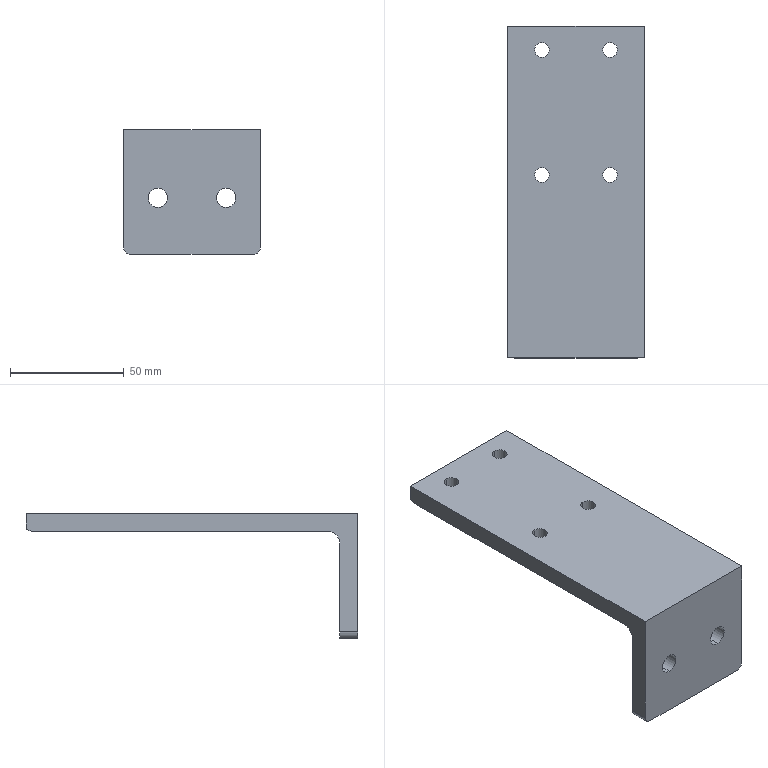Part | SolidWorks | features HoleWzd 2, ICE 2, 3DProfileFeature 1, Fillet 1, WeldMemberFeat 1, WeldmentFeature 1 | 1 solid | 24 faces | box 60 x 146 x 55 mm | volume 90878 mm3 | cylinder 16 | plane 8 | commonest cylinder face diameters 6.5 x8 8.5 x4 6 x2 10 x1 16 x1
STEP:
#1=CARTESIAN_POINT('',(15.,0.,-34.25));
#2=VERTEX_POINT('',#1);
#3=CARTESIAN_POINT('',(15.,0.,-25.75));
#4=VERTEX_POINT('',#3);
#5=CARTESIAN_POINT('',(15.,0.,-30.));
#6=DIRECTION('',(0.,1.,0.));
#7=DIRECTION('',(0.,0.,1.));
#8=AXIS2_PLACEMENT_3D('',#5,#6,#7);
#9=CIRCLE('',#8,4.25);
#10=EDGE_CURVE('',#2,#4,#9,.T.);
#11=ORIENTED_EDGE('',*,*,#10,.F.);
#12=CARTESIAN_POINT('',(15.,8.,-34.25));
#13=VERTEX_POINT('',#12);
#14=CARTESIAN_POINT('',(15.,8.,-34.25));
#15=DIRECTION('',(0.,1.,0.));
#16=VECTOR('',#15,1000.);
#17=LINE('',#14,#16);
#18=EDGE_CURVE('',#2,#13,#17,.T.);
#19=ORIENTED_EDGE('',*,*,#18,.T.);
#20=CARTESIAN_POINT('',(15.,8.,-25.75));
#21=VERTEX_POINT('',#20);
#22=CARTESIAN_POINT('',(15.,8.,-30.));
#23=DIRECTION('',(0.,1.,0.));
#24=DIRECTION('',(0.,0.,1.));
#25=AXIS2_PLACEMENT_3D('',#22,#23,#24);
#26=CIRCLE('',#25,4.25);
#27=EDGE_CURVE('',#13,#21,#26,.T.);
#28=ORIENTED_EDGE('',*,*,#27,.T.);
#29=CARTESIAN_POINT('',(15.,8.,-25.75));
#30=DIRECTION('',(0.,1.,0.));
#31=VECTOR('',#30,1000.);
#32=LINE('',#29,#31);
#33=EDGE_CURVE('',#4,#21,#32,.T.);
#34=ORIENTED_EDGE('',*,*,#33,.F.);
#35=EDGE_LOOP('',(#11,#19,#28,#34));
#36=FACE_OUTER_BOUND('',#35,.T.);
#37=CARTESIAN_POINT('',(15.,8.,-30.));
#38=DIRECTION('',(0.,1.,0.));
#39=DIRECTION('',(0.,0.,1.));
#40=AXIS2_PLACEMENT_3D('',#37,#38,#39);
#41=CYLINDRICAL_SURFACE('',#40,4.25);
#42=ADVANCED_FACE('',(#36),#41,.F.);
#43=CARTESIAN_POINT('',(45.,0.,-34.25));
#44=VERTEX_POINT('',#43);
#45=CARTESIAN_POINT('',(45.,0.,-25.75));
#46=VERTEX_POINT('',#45);
#47=CARTESIAN_POINT('',(45.,0.,-30.));
#48=DIRECTION('',(0.,1.,0.));
#49=DIRECTION('',(0.,0.,1.));
#50=AXIS2_PLACEMENT_3D('',#47,#48,#49);
#51=CIRCLE('',#50,4.25);
#52=EDGE_CURVE('',#44,#46,#51,.T.);
#53=ORIENTED_EDGE('',*,*,#52,.F.);
#54=CARTESIAN_POINT('',(45.,8.,-34.25));
#55=VERTEX_POINT('',#54);
#56=CARTESIAN_POINT('',(45.,8.,-34.25));
#57=DIRECTION('',(0.,1.,0.));
#58=VECTOR('',#57,1000.);
#59=LINE('',#56,#58);
#60=EDGE_CURVE('',#44,#55,#59,.T.);
#61=ORIENTED_EDGE('',*,*,#60,.T.);
#62=CARTESIAN_POINT('',(45.,8.,-25.75));
#63=VERTEX_POINT('',#62);
#64=CARTESIAN_POINT('',(45.,8.,-30.));
#65=DIRECTION('',(0.,1.,0.));
#66=DIRECTION('',(0.,0.,1.));
#67=AXIS2_PLACEMENT_3D('',#64,#65,#66);
#68=CIRCLE('',#67,4.25);
#69=EDGE_CURVE('',#55,#63,#68,.T.);
#70=ORIENTED_EDGE('',*,*,#69,.T.);
#71=CARTESIAN_POINT('',(45.,8.,-25.75));
#72=DIRECTION('',(0.,1.,0.));
#73=VECTOR('',#72,1000.);
#74=LINE('',#71,#73);
#75=EDGE_CURVE('',#46,#63,#74,.T.);
#76=ORIENTED_EDGE('',*,*,#75,.F.);
#77=EDGE_LOOP('',(#53,#61,#70,#76));
#78=FACE_OUTER_BOUND('',#77,.T.);
#79=CARTESIAN_POINT('',(45.,8.,-30.));
#80=DIRECTION('',(0.,1.,0.));
#81=DIRECTION('',(0.,0.,1.));
#82=AXIS2_PLACEMENT_3D('',#79,#80,#81);
#83=CYLINDRICAL_SURFACE('',#82,4.25);
#84=ADVANCED_FACE('',(#78),#83,.F.);
#85=CARTESIAN_POINT('',(45.,132.25,0.));
#86=VERTEX_POINT('',#85);
#87=CARTESIAN_POINT('',(45.,138.75,0.));
#88=VERTEX_POINT('',#87);
#89=CARTESIAN_POINT('',(45.,135.5,0.));
#90=DIRECTION('',(0.,0.,-1.));
#91=DIRECTION('',(0.,1.,0.));
#92=AXIS2_PLACEMENT_3D('',#89,#90,#91);
#93=CIRCLE('',#92,3.25);
#94=EDGE_CURVE('',#86,#88,#93,.T.);
#95=ORIENTED_EDGE('',*,*,#94,.F.);
#96=CARTESIAN_POINT('',(45.,132.25,-8.));
#97=VERTEX_POINT('',#96);
#98=CARTESIAN_POINT('',(45.,132.25,-8.));
#99=DIRECTION('',(0.,0.,-1.));
#100=VECTOR('',#99,1000.);
#101=LINE('',#98,#100);
#102=EDGE_CURVE('',#86,#97,#101,.T.);
#103=ORIENTED_EDGE('',*,*,#102,.T.);
#104=CARTESIAN_POINT('',(45.,138.75,-8.));
#105=VERTEX_POINT('',#104);
#106=CARTESIAN_POINT('',(45.,135.5,-8.));
#107=DIRECTION('',(0.,0.,-1.));
#108=DIRECTION('',(0.,1.,0.));
#109=AXIS2_PLACEMENT_3D('',#106,#107,#108);
#110=CIRCLE('',#109,3.25);
#111=EDGE_CURVE('',#97,#105,#110,.T.);
#112=ORIENTED_EDGE('',*,*,#111,.T.);
#113=CARTESIAN_POINT('',(45.,138.75,-8.));
#114=DIRECTION('',(0.,0.,-1.));
#115=VECTOR('',#114,1000.);
#116=LINE('',#113,#115);
#117=EDGE_CURVE('',#88,#105,#116,.T.);
#118=ORIENTED_EDGE('',*,*,#117,.F.);
#119=EDGE_LOOP('',(#95,#103,#112,#118));
#120=FACE_OUTER_BOUND('',#119,.T.);
#121=CARTESIAN_POINT('',(45.,135.5,-8.));
#122=DIRECTION('',(0.,0.,-1.));
#123=DIRECTION('',(0.,1.,0.));
#124=AXIS2_PLACEMENT_3D('',#121,#122,#123);
#125=CYLINDRICAL_SURFACE('',#124,3.25);
#126=ADVANCED_FACE('',(#120),#125,.F.);
#127=CARTESIAN_POINT('',(15.,132.25,0.));
#128=VERTEX_POINT('',#127);
#129=CARTESIAN_POINT('',(15.,138.75,0.));
#130=VERTEX_POINT('',#129);
#131=CARTESIAN_POINT('',(15.,135.5,0.));
#132=DIRECTION('',(0.,0.,-1.));
#133=DIRECTION('',(0.,1.,0.));
#134=AXIS2_PLACEMENT_3D('',#131,#132,#133);
#135=CIRCLE('',#134,3.25);
#136=EDGE_CURVE('',#128,#130,#135,.T.);
#137=ORIENTED_EDGE('',*,*,#136,.F.);
#138=CARTESIAN_POINT('',(15.,132.25,-8.));
#139=VERTEX_POINT('',#138);
#140=CARTESIAN_POINT('',(15.,132.25,-8.));
#141=DIRECTION('',(0.,0.,-1.));
#142=VECTOR('',#141,1000.);
#143=LINE('',#140,#142);
#144=EDGE_CURVE('',#128,#139,#143,.T.);
#145=ORIENTED_EDGE('',*,*,#144,.T.);
#146=CARTESIAN_POINT('',(15.,138.75,-8.));
#147=VERTEX_POINT('',#146);
#148=CARTESIAN_POINT('',(15.,135.5,-8.));
#149=DIRECTION('',(0.,0.,-1.));
#150=DIRECTION('',(0.,1.,0.));
#151=AXIS2_PLACEMENT_3D('',#148,#149,#150);
#152=CIRCLE('',#151,3.25);
#153=EDGE_CURVE('',#139,#147,#152,.T.);
#154=ORIENTED_EDGE('',*,*,#153,.T.);
#155=CARTESIAN_POINT('',(15.,138.75,-8.));
#156=DIRECTION('',(0.,0.,-1.));
#157=VECTOR('',#156,1000.);
#158=LINE('',#155,#157);
#159=EDGE_CURVE('',#130,#147,#158,.T.);
#160=ORIENTED_EDGE('',*,*,#159,.F.);
#161=EDGE_LOOP('',(#137,#145,#154,#160));
#162=FACE_OUTER_BOUND('',#161,.T.);
#163=CARTESIAN_POINT('',(15.,135.5,-8.));
#164=DIRECTION('',(0.,0.,-1.));
#165=DIRECTION('',(0.,1.,0.));
#166=AXIS2_PLACEMENT_3D('',#163,#164,#165);
#167=CYLINDRICAL_SURFACE('',#166,3.25);
#168=ADVANCED_FACE('',(#162),#167,.F.);
#169=CARTESIAN_POINT('',(45.,77.25,0.));
#170=VERTEX_POINT('',#169);
#171=CARTESIAN_POINT('',(45.,83.75,0.));
#172=VERTEX_POINT('',#171);
#173=CARTESIAN_POINT('',(45.,80.5,0.));
#174=DIRECTION('',(0.,0.,-1.));
#175=DIRECTION('',(0.,1.,0.));
#176=AXIS2_PLACEMENT_3D('',#173,#174,#175);
#177=CIRCLE('',#176,3.25);
#178=EDGE_CURVE('',#170,#172,#177,.T.);
#179=ORIENTED_EDGE('',*,*,#178,.F.);
#180=CARTESIAN_POINT('',(45.,77.25,-8.));
#181=VERTEX_POINT('',#180);
#182=CARTESIAN_POINT('',(45.,77.25,-8.));
#183=DIRECTION('',(0.,0.,-1.));
#184=VECTOR('',#183,1000.);
#185=LINE('',#182,#184);
#186=EDGE_CURVE('',#170,#181,#185,.T.);
#187=ORIENTED_EDGE('',*,*,#186,.T.);
#188=CARTESIAN_POINT('',(45.,83.75,-8.));
#189=VERTEX_POINT('',#188);
#190=CARTESIAN_POINT('',(45.,80.5,-8.));
#191=DIRECTION('',(0.,0.,-1.));
#192=DIRECTION('',(0.,1.,0.));
#193=AXIS2_PLACEMENT_3D('',#190,#191,#192);
#194=CIRCLE('',#193,3.25);
#195=EDGE_CURVE('',#181,#189,#194,.T.);
#196=ORIENTED_EDGE('',*,*,#195,.T.);
#197=CARTESIAN_POINT('',(45.,83.75,-8.));
#198=DIRECTION('',(0.,0.,-1.));
#199=VECTOR('',#198,1000.);
#200=LINE('',#197,#199);
#201=EDGE_CURVE('',#172,#189,#200,.T.);
#202=ORIENTED_EDGE('',*,*,#201,.F.);
#203=EDGE_LOOP('',(#179,#187,#196,#202));
#204=FACE_OUTER_BOUND('',#203,.T.);
#205=CARTESIAN_POINT('',(45.,80.5,-8.));
#206=DIRECTION('',(0.,0.,-1.));
#207=DIRECTION('',(0.,1.,0.));
#208=AXIS2_PLACEMENT_3D('',#205,#206,#207);
#209=CYLINDRICAL_SURFACE('',#208,3.25);
#210=ADVANCED_FACE('',(#204),#209,.F.);
#211=CARTESIAN_POINT('',(15.,77.25,0.));
#212=VERTEX_POINT('',#211);
#213=CARTESIAN_POINT('',(15.,83.75,0.));
#214=VERTEX_POINT('',#213);
#215=CARTESIAN_POINT('',(15.,80.5,0.));
#216=DIRECTION('',(0.,0.,-1.));
#217=DIRECTION('',(0.,1.,0.));
#218=AXIS2_PLACEMENT_3D('',#215,#216,#217);
#219=CIRCLE('',#218,3.25);
#220=EDGE_CURVE('',#212,#214,#219,.T.);
#221=ORIENTED_EDGE('',*,*,#220,.F.);
#222=CARTESIAN_POINT('',(15.,77.25,-8.));
#223=VERTEX_POINT('',#222);
#224=CARTESIAN_POINT('',(15.,77.25,-8.));
#225=DIRECTION('',(0.,0.,-1.));
#226=VECTOR('',#225,1000.);
#227=LINE('',#224,#226);
#228=EDGE_CURVE('',#212,#223,#227,.T.);
#229=ORIENTED_EDGE('',*,*,#228,.T.);
#230=CARTESIAN_POINT('',(15.,83.75,-8.));
#231=VERTEX_POINT('',#230);
#232=CARTESIAN_POINT('',(15.,80.5,-8.));
#233=DIRECTION('',(0.,0.,-1.));
#234=DIRECTION('',(0.,1.,0.));
#235=AXIS2_PLACEMENT_3D('',#232,#233,#234);
#236=CIRCLE('',#235,3.25);
#237=EDGE_CURVE('',#223,#231,#236,.T.);
#238=ORIENTED_EDGE('',*,*,#237,.T.);
#239=CARTESIAN_POINT('',(15.,83.75,-8.));
#240=DIRECTION('',(0.,0.,-1.));
#241=VECTOR('',#240,1000.);
#242=LINE('',#239,#241);
#243=EDGE_CURVE('',#214,#231,#242,.T.);
#244=ORIENTED_EDGE('',*,*,#243,.F.);
#245=EDGE_LOOP('',(#221,#229,#238,#244));
#246=FACE_OUTER_BOUND('',#245,.T.);
#247=CARTESIAN_POINT('',(15.,80.5,-8.));
#248=DIRECTION('',(0.,0.,-1.));
#249=DIRECTION('',(0.,1.,0.));
#250=AXIS2_PLACEMENT_3D('',#247,#248,#249);
#251=CYLINDRICAL_SURFACE('',#250,3.25);
#252=ADVANCED_FACE('',(#246),#251,.F.);
#253=CARTESIAN_POINT('',(45.,135.5,-8.));
#254=DIRECTION('',(0.,0.,-1.));
#255=DIRECTION('',(0.,1.,0.));
#256=AXIS2_PLACEMENT_3D('',#253,#254,#255);
#257=CIRCLE('',#256,3.25);
#258=EDGE_CURVE('',#105,#97,#257,.T.);
#259=ORIENTED_EDGE('',*,*,#258,.F.);
#260=ORIENTED_EDGE('',*,*,#111,.F.);
#261=EDGE_LOOP('',(#259,#260));
#262=FACE_BOUND('',#261,.T.);
#263=CARTESIAN_POINT('',(45.,80.5,-8.));
#264=DIRECTION('',(0.,0.,-1.));
#265=DIRECTION('',(0.,1.,0.));
#266=AXIS2_PLACEMENT_3D('',#263,#264,#265);
#267=CIRCLE('',#266,3.25);
#268=EDGE_CURVE('',#189,#181,#267,.T.);
#269=ORIENTED_EDGE('',*,*,#268,.F.);
#270=ORIENTED_EDGE('',*,*,#195,.F.);
#271=EDGE_LOOP('',(#269,#270));
#272=FACE_BOUND('',#271,.T.);
#273=CARTESIAN_POINT('',(15.,80.5,-8.));
#274=DIRECTION('',(0.,0.,-1.));
#275=DIRECTION('',(0.,1.,0.));
#276=AXIS2_PLACEMENT_3D('',#273,#274,#275);
#277=CIRCLE('',#276,3.25);
#278=EDGE_CURVE('',#231,#223,#277,.T.);
#279=ORIENTED_EDGE('',*,*,#278,.F.);
#280=ORIENTED_EDGE('',*,*,#237,.F.);
#281=EDGE_LOOP('',(#279,#280));
#282=FACE_BOUND('',#281,.T.);
#283=CARTESIAN_POINT('',(0.,13.,-8.));
#284=VERTEX_POINT('',#283);
#285=CARTESIAN_POINT('',(0.,142.,-8.));
#286=VERTEX_POINT('',#285);
#287=CARTESIAN_POINT('',(0.,142.,-8.));
#288=DIRECTION('',(0.,1.,0.));
#289=VECTOR('',#288,1000.);
#290=LINE('',#287,#289);
#291=EDGE_CURVE('',#284,#286,#290,.T.);
#292=ORIENTED_EDGE('',*,*,#291,.T.);
#293=CARTESIAN_POINT('',(60.,142.,-8.));
#294=VERTEX_POINT('',#293);
#295=CARTESIAN_POINT('',(60.,142.,-8.));
#296=DIRECTION('',(-1.,0.,0.));
#297=VECTOR('',#296,1000.);
#298=LINE('',#295,#297);
#299=EDGE_CURVE('',#294,#286,#298,.T.);
#300=ORIENTED_EDGE('',*,*,#299,.F.);
#301=CARTESIAN_POINT('',(60.,13.,-8.));
#302=VERTEX_POINT('',#301);
#303=CARTESIAN_POINT('',(60.,142.,-8.));
#304=DIRECTION('',(0.,1.,0.));
#305=VECTOR('',#304,1000.);
#306=LINE('',#303,#305);
#307=EDGE_CURVE('',#302,#294,#306,.T.);
#308=ORIENTED_EDGE('',*,*,#307,.F.);
#309=CARTESIAN_POINT('',(60.,13.,-8.));
#310=DIRECTION('',(-1.,0.,0.));
#311=VECTOR('',#310,1000.);
#312=LINE('',#309,#311);
#313=EDGE_CURVE('',#302,#284,#312,.T.);
#314=ORIENTED_EDGE('',*,*,#313,.T.);
#315=EDGE_LOOP('',(#292,#300,#308,#314));
#316=FACE_OUTER_BOUND('',#315,.T.);
#317=CARTESIAN_POINT('',(15.,135.5,-8.));
#318=DIRECTION('',(0.,0.,-1.));
#319=DIRECTION('',(0.,1.,0.));
#320=AXIS2_PLACEMENT_3D('',#317,#318,#319);
#321=CIRCLE('',#320,3.25);
#322=EDGE_CURVE('',#147,#139,#321,.T.);
#323=ORIENTED_EDGE('',*,*,#322,.F.);
#324=ORIENTED_EDGE('',*,*,#153,.F.);
#325=EDGE_LOOP('',(#323,#324));
#326=FACE_BOUND('',#325,.T.);
#327=CARTESIAN_POINT('',(60.,142.,-8.));
#328=DIRECTION('',(0.,0.,1.));
#329=DIRECTION('',(0.,-1.,0.));
#330=AXIS2_PLACEMENT_3D('',#327,#328,#329);
#331=PLANE('',#330);
#332=ADVANCED_FACE('',(#262,#272,#282,#316,#326),#331,.F.);
#333=CARTESIAN_POINT('',(15.,0.,-30.));
#334=DIRECTION('',(0.,1.,0.));
#335=DIRECTION('',(0.,0.,1.));
#336=AXIS2_PLACEMENT_3D('',#333,#334,#335);
#337=CIRCLE('',#336,4.25);
#338=EDGE_CURVE('',#4,#2,#337,.T.);
#339=ORIENTED_EDGE('',*,*,#338,.T.);
#340=ORIENTED_EDGE('',*,*,#10,.T.);
#341=EDGE_LOOP('',(#339,#340));
#342=FACE_BOUND('',#341,.T.);
#343=CARTESIAN_POINT('',(45.,0.,-30.));
#344=DIRECTION('',(0.,1.,0.));
#345=DIRECTION('',(0.,0.,1.));
#346=AXIS2_PLACEMENT_3D('',#343,#344,#345);
#347=CIRCLE('',#346,4.25);
#348=EDGE_CURVE('',#46,#44,#347,.T.);
#349=ORIENTED_EDGE('',*,*,#348,.T.);
#350=ORIENTED_EDGE('',*,*,#52,.T.);
#351=EDGE_LOOP('',(#349,#350));
#352=FACE_BOUND('',#351,.T.);
#353=CARTESIAN_POINT('',(0.,0.,0.));
#354=VERTEX_POINT('',#353);
#355=CARTESIAN_POINT('',(0.,0.,-52.));
#356=VERTEX_POINT('',#355);
#357=CARTESIAN_POINT('',(0.,0.,-70.));
#358=DIRECTION('',(0.,0.,-1.));
#359=VECTOR('',#358,1000.);
#360=LINE('',#357,#359);
#361=EDGE_CURVE('',#354,#356,#360,.T.);
#362=ORIENTED_EDGE('',*,*,#361,.T.);
#363=CARTESIAN_POINT('',(3.,0.,-55.));
#364=VERTEX_POINT('',#363);
#365=CARTESIAN_POINT('',(3.,0.,-52.));
#366=DIRECTION('',(0.,-1.,0.));
#367=DIRECTION('',(0.,0.,1.));
#368=AXIS2_PLACEMENT_3D('',#365,#366,#367);
#369=CIRCLE('',#368,3.);
#370=EDGE_CURVE('',#356,#364,#369,.T.);
#371=ORIENTED_EDGE('',*,*,#370,.T.);
#372=CARTESIAN_POINT('',(57.,0.,-55.));
#373=VERTEX_POINT('',#372);
#374=CARTESIAN_POINT('',(0.,0.,-55.));
#375=DIRECTION('',(-1.,0.,0.));
#376=VECTOR('',#375,1000.);
#377=LINE('',#374,#376);
#378=EDGE_CURVE('',#373,#364,#377,.T.);
#379=ORIENTED_EDGE('',*,*,#378,.F.);
#380=CARTESIAN_POINT('',(60.,0.,-52.));
#381=VERTEX_POINT('',#380);
#382=CARTESIAN_POINT('',(57.,0.,-52.));
#383=DIRECTION('',(0.,-1.,0.));
#384=DIRECTION('',(0.,0.,1.));
#385=AXIS2_PLACEMENT_3D('',#382,#383,#384);
#386=CIRCLE('',#385,3.);
#387=EDGE_CURVE('',#373,#381,#386,.T.);
#388=ORIENTED_EDGE('',*,*,#387,.T.);
#389=CARTESIAN_POINT('',(60.,0.,0.));
#390=VERTEX_POINT('',#389);
#391=CARTESIAN_POINT('',(60.,0.,-70.));
#392=DIRECTION('',(0.,0.,-1.));
#393=VECTOR('',#392,1000.);
#394=LINE('',#391,#393);
#395=EDGE_CURVE('',#390,#381,#394,.T.);
#396=ORIENTED_EDGE('',*,*,#395,.F.);
#397=CARTESIAN_POINT('',(60.,0.,0.));
#398=DIRECTION('',(-1.,0.,0.));
#399=VECTOR('',#398,1000.);
#400=LINE('',#397,#399);
#401=EDGE_CURVE('',#390,#354,#400,.T.);
#402=ORIENTED_EDGE('',*,*,#401,.T.);
#403=EDGE_LOOP('',(#362,#371,#379,#388,#396,#402));
#404=FACE_OUTER_BOUND('',#403,.T.);
#405=CARTESIAN_POINT('',(60.,0.,-70.));
#406=DIRECTION('',(0.,1.,0.));
#407=DIRECTION('',(0.,0.,1.));
#408=AXIS2_PLACEMENT_3D('',#405,#406,#407);
#409=PLANE('',#408);
#410=ADVANCED_FACE('',(#342,#352,#404),#409,.F.);
#411=CARTESIAN_POINT('',(15.,8.,-30.));
#412=DIRECTION('',(0.,1.,0.));
#413=DIRECTION('',(0.,0.,1.));
#414=AXIS2_PLACEMENT_3D('',#411,#412,#413);
#415=CIRCLE('',#414,4.25);
#416=EDGE_CURVE('',#21,#13,#415,.T.);
#417=ORIENTED_EDGE('',*,*,#416,.F.);
#418=ORIENTED_EDGE('',*,*,#27,.F.);
#419=EDGE_LOOP('',(#417,#418));
#420=FACE_BOUND('',#419,.T.);
#421=CARTESIAN_POINT('',(45.,8.,-30.));
#422=DIRECTION('',(0.,1.,0.));
#423=DIRECTION('',(0.,0.,1.));
#424=AXIS2_PLACEMENT_3D('',#421,#422,#423);
#425=CIRCLE('',#424,4.25);
#426=EDGE_CURVE('',#63,#55,#425,.T.);
#427=ORIENTED_EDGE('',*,*,#426,.F.);
#428=ORIENTED_EDGE('',*,*,#69,.F.);
#429=EDGE_LOOP('',(#427,#428));
#430=FACE_BOUND('',#429,.T.);
#431=CARTESIAN_POINT('',(57.,8.,-55.));
#432=VERTEX_POINT('',#431);
#433=CARTESIAN_POINT('',(3.,8.,-55.));
#434=VERTEX_POINT('',#433);
#435=CARTESIAN_POINT('',(60.,8.,-55.));
#436=DIRECTION('',(-1.,0.,0.));
#437=VECTOR('',#436,1000.);
#438=LINE('',#435,#437);
#439=EDGE_CURVE('',#432,#434,#438,.T.);
#440=ORIENTED_EDGE('',*,*,#439,.T.);
#441=CARTESIAN_POINT('',(0.,8.,-52.));
#442=VERTEX_POINT('',#441);
#443=CARTESIAN_POINT('',(3.,8.,-52.));
#444=DIRECTION('',(0.,1.,0.));
#445=DIRECTION('',(0.,0.,-1.));
#446=AXIS2_PLACEMENT_3D('',#443,#444,#445);
#447=CIRCLE('',#446,3.);
#448=EDGE_CURVE('',#434,#442,#447,.T.);
#449=ORIENTED_EDGE('',*,*,#448,.T.);
#450=CARTESIAN_POINT('',(0.,8.,-13.));
#451=VERTEX_POINT('',#450);
#452=CARTESIAN_POINT('',(0.,8.,-13.));
#453=DIRECTION('',(0.,0.,1.));
#454=VECTOR('',#453,1000.);
#455=LINE('',#452,#454);
#456=EDGE_CURVE('',#442,#451,#455,.T.);
#457=ORIENTED_EDGE('',*,*,#456,.T.);
#458=CARTESIAN_POINT('',(60.,8.,-13.));
#459=VERTEX_POINT('',#458);
#460=CARTESIAN_POINT('',(60.,8.,-13.));
#461=DIRECTION('',(-1.,0.,0.));
#462=VECTOR('',#461,1000.);
#463=LINE('',#460,#462);
#464=EDGE_CURVE('',#459,#451,#463,.T.);
#465=ORIENTED_EDGE('',*,*,#464,.F.);
#466=CARTESIAN_POINT('',(60.,8.,-52.));
#467=VERTEX_POINT('',#466);
#468=CARTESIAN_POINT('',(60.,8.,-13.));
#469=DIRECTION('',(0.,0.,1.));
#470=VECTOR('',#469,1000.);
#471=LINE('',#468,#470);
#472=EDGE_CURVE('',#467,#459,#471,.T.);
#473=ORIENTED_EDGE('',*,*,#472,.F.);
#474=CARTESIAN_POINT('',(57.,8.,-52.));
#475=DIRECTION('',(0.,1.,0.));
#476=DIRECTION('',(0.,0.,-1.));
#477=AXIS2_PLACEMENT_3D('',#474,#475,#476);
#478=CIRCLE('',#477,3.);
#479=EDGE_CURVE('',#467,#432,#478,.T.);
#480=ORIENTED_EDGE('',*,*,#479,.T.);
#481=EDGE_LOOP('',(#440,#449,#457,#465,#473,#480));
#482=FACE_OUTER_BOUND('',#481,.T.);
#483=CARTESIAN_POINT('',(60.,8.,-13.));
#484=DIRECTION('',(0.,-1.,0.));
#485=DIRECTION('',(0.,0.,-1.));
#486=AXIS2_PLACEMENT_3D('',#483,#484,#485);
#487=PLANE('',#486);
#488=ADVANCED_FACE('',(#420,#430,#482),#487,.F.);
#489=CARTESIAN_POINT('',(0.,13.,-13.));
#490=DIRECTION('',(-1.,0.,0.));
#491=DIRECTION('',(0.,0.,1.));
#492=AXIS2_PLACEMENT_3D('',#489,#490,#491);
#493=CIRCLE('',#492,5.);
#494=EDGE_CURVE('',#451,#284,#493,.T.);
#495=ORIENTED_EDGE('',*,*,#494,.T.);
#496=ORIENTED_EDGE('',*,*,#313,.F.);
#497=CARTESIAN_POINT('',(60.,13.,-13.));
#498=DIRECTION('',(-1.,0.,0.));
#499=DIRECTION('',(0.,0.,1.));
#500=AXIS2_PLACEMENT_3D('',#497,#498,#499);
#501=CIRCLE('',#500,5.);
#502=EDGE_CURVE('',#459,#302,#501,.T.);
#503=ORIENTED_EDGE('',*,*,#502,.F.);
#504=ORIENTED_EDGE('',*,*,#464,.T.);
#505=EDGE_LOOP('',(#495,#496,#503,#504));
#506=FACE_OUTER_BOUND('',#505,.T.);
#507=CARTESIAN_POINT('',(60.,13.,-13.));
#508=DIRECTION('',(-1.,0.,0.));
#509=DIRECTION('',(0.,0.,1.));
#510=AXIS2_PLACEMENT_3D('',#507,#508,#509);
#511=CYLINDRICAL_SURFACE('',#510,5.);
#512=ADVANCED_FACE('',(#506),#511,.F.);
#513=CARTESIAN_POINT('',(0.,146.,-6.928));
#514=VERTEX_POINT('',#513);
#515=CARTESIAN_POINT('',(0.,142.,0.));
#516=DIRECTION('',(1.,0.,0.));
#517=DIRECTION('',(0.,0.,1.));
#518=AXIS2_PLACEMENT_3D('',#515,#516,#517);
#519=CIRCLE('',#518,8.);
#520=EDGE_CURVE('',#286,#514,#519,.T.);
#521=ORIENTED_EDGE('',*,*,#520,.T.);
#522=CARTESIAN_POINT('',(60.,146.,-6.928));
#523=VERTEX_POINT('',#522);
#524=CARTESIAN_POINT('',(60.,146.,-6.928));
#525=DIRECTION('',(1.,0.,0.));
#526=VECTOR('',#525,1000.);
#527=LINE('',#524,#526);
#528=EDGE_CURVE('',#514,#523,#527,.T.);
#529=ORIENTED_EDGE('',*,*,#528,.T.);
#530=CARTESIAN_POINT('',(60.,142.,0.));
#531=DIRECTION('',(1.,0.,0.));
#532=DIRECTION('',(0.,0.,1.));
#533=AXIS2_PLACEMENT_3D('',#530,#531,#532);
#534=CIRCLE('',#533,8.);
#535=EDGE_CURVE('',#294,#523,#534,.T.);
#536=ORIENTED_EDGE('',*,*,#535,.F.);
#537=ORIENTED_EDGE('',*,*,#299,.T.);
#538=EDGE_LOOP('',(#521,#529,#536,#537));
#539=FACE_OUTER_BOUND('',#538,.T.);
#540=CARTESIAN_POINT('',(60.,142.,0.));
#541=DIRECTION('',(-1.,0.,0.));
#542=DIRECTION('',(0.,0.,1.));
#543=AXIS2_PLACEMENT_3D('',#540,#541,#542);
#544=CYLINDRICAL_SURFACE('',#543,8.);
#545=ADVANCED_FACE('',(#539),#544,.T.);
#546=CARTESIAN_POINT('',(45.,135.5,0.));
#547=DIRECTION('',(0.,0.,-1.));
#548=DIRECTION('',(0.,1.,0.));
#549=AXIS2_PLACEMENT_3D('',#546,#547,#548);
#550=CIRCLE('',#549,3.25);
#551=EDGE_CURVE('',#88,#86,#550,.T.);
#552=ORIENTED_EDGE('',*,*,#551,.T.);
#553=ORIENTED_EDGE('',*,*,#94,.T.);
#554=EDGE_LOOP('',(#552,#553));
#555=FACE_BOUND('',#554,.T.);
#556=CARTESIAN_POINT('',(15.,135.5,0.));
#557=DIRECTION('',(0.,0.,-1.));
#558=DIRECTION('',(0.,1.,0.));
#559=AXIS2_PLACEMENT_3D('',#556,#557,#558);
#560=CIRCLE('',#559,3.25);
#561=EDGE_CURVE('',#130,#128,#560,.T.);
#562=ORIENTED_EDGE('',*,*,#561,.T.);
#563=ORIENTED_EDGE('',*,*,#136,.T.);
#564=EDGE_LOOP('',(#562,#563));
#565=FACE_BOUND('',#564,.T.);
#566=CARTESIAN_POINT('',(45.,80.5,0.));
#567=DIRECTION('',(0.,0.,-1.));
#568=DIRECTION('',(0.,1.,0.));
#569=AXIS2_PLACEMENT_3D('',#566,#567,#568);
#570=CIRCLE('',#569,3.25);
#571=EDGE_CURVE('',#172,#170,#570,.T.);
#572=ORIENTED_EDGE('',*,*,#571,.T.);
#573=ORIENTED_EDGE('',*,*,#178,.T.);
#574=EDGE_LOOP('',(#572,#573));
#575=FACE_BOUND('',#574,.T.);
#576=CARTESIAN_POINT('',(15.,80.5,0.));
#577=DIRECTION('',(0.,0.,-1.));
#578=DIRECTION('',(0.,1.,0.));
#579=AXIS2_PLACEMENT_3D('',#576,#577,#578);
#580=CIRCLE('',#579,3.25);
#581=EDGE_CURVE('',#214,#212,#580,.T.);
#582=ORIENTED_EDGE('',*,*,#581,.T.);
#583=ORIENTED_EDGE('',*,*,#220,.T.);
#584=EDGE_LOOP('',(#582,#583));
#585=FACE_BOUND('',#584,.T.);
#586=CARTESIAN_POINT('',(60.,146.,0.));
#587=VERTEX_POINT('',#586);
#588=CARTESIAN_POINT('',(60.,0.,0.));
#589=DIRECTION('',(0.,-1.,0.));
#590=VECTOR('',#589,1000.);
#591=LINE('',#588,#590);
#592=EDGE_CURVE('',#587,#390,#591,.T.);
#593=ORIENTED_EDGE('',*,*,#592,.F.);
#594=CARTESIAN_POINT('',(0.,146.,0.));
#595=VERTEX_POINT('',#594);
#596=CARTESIAN_POINT('',(60.,146.,0.));
#597=DIRECTION('',(1.,0.,0.));
#598=VECTOR('',#597,1000.);
#599=LINE('',#596,#598);
#600=EDGE_CURVE('',#595,#587,#599,.T.);
#601=ORIENTED_EDGE('',*,*,#600,.F.);
#602=CARTESIAN_POINT('',(0.,0.,0.));
#603=DIRECTION('',(0.,-1.,0.));
#604=VECTOR('',#603,1000.);
#605=LINE('',#602,#604);
#606=EDGE_CURVE('',#595,#354,#605,.T.);
#607=ORIENTED_EDGE('',*,*,#606,.T.);
#608=ORIENTED_EDGE('',*,*,#401,.F.);
#609=EDGE_LOOP('',(#593,#601,#607,#608));
#610=FACE_OUTER_BOUND('',#609,.T.);
#611=CARTESIAN_POINT('',(60.,0.,0.));
#612=DIRECTION('',(0.,0.,-1.));
#613=DIRECTION('',(-1.,0.,0.));
#614=AXIS2_PLACEMENT_3D('',#611,#612,#613);
#615=PLANE('',#614);
#616=ADVANCED_FACE('',(#555,#565,#575,#585,#610),#615,.F.);
#617=ORIENTED_EDGE('',*,*,#395,.T.);
#618=CARTESIAN_POINT('',(60.,142.,-52.));
#619=DIRECTION('',(0.,1.,0.));
#620=VECTOR('',#619,1000.);
#621=LINE('',#618,#620);
#622=EDGE_CURVE('',#381,#467,#621,.T.);
#623=ORIENTED_EDGE('',*,*,#622,.T.);
#624=ORIENTED_EDGE('',*,*,#472,.T.);
#625=ORIENTED_EDGE('',*,*,#502,.T.);
#626=ORIENTED_EDGE('',*,*,#307,.T.);
#627=ORIENTED_EDGE('',*,*,#535,.T.);
#628=CARTESIAN_POINT('',(60.,146.,-55.));
#629=DIRECTION('',(0.,0.,1.));
#630=VECTOR('',#629,1000.);
#631=LINE('',#628,#630);
#632=EDGE_CURVE('',#523,#587,#631,.T.);
#633=ORIENTED_EDGE('',*,*,#632,.T.);
#634=ORIENTED_EDGE('',*,*,#592,.T.);
#635=EDGE_LOOP('',(#617,#623,#624,#625,#626,#627,#633,#634));
#636=FACE_OUTER_BOUND('',#635,.T.);
#637=CARTESIAN_POINT('',(60.,142.,0.));
#638=DIRECTION('',(-1.,0.,0.));
#639=DIRECTION('',(0.,0.,1.));
#640=AXIS2_PLACEMENT_3D('',#637,#638,#639);
#641=PLANE('',#640);
#642=ADVANCED_FACE('',(#636),#641,.F.);
#643=ORIENTED_EDGE('',*,*,#456,.F.);
#644=CARTESIAN_POINT('',(0.,0.,-52.));
#645=DIRECTION('',(0.,-1.,0.));
#646=VECTOR('',#645,1000.);
#647=LINE('',#644,#646);
#648=EDGE_CURVE('',#442,#356,#647,.T.);
#649=ORIENTED_EDGE('',*,*,#648,.T.);
#650=ORIENTED_EDGE('',*,*,#361,.F.);
#651=ORIENTED_EDGE('',*,*,#606,.F.);
#652=CARTESIAN_POINT('',(0.,146.,0.));
#653=DIRECTION('',(0.,0.,1.));
#654=VECTOR('',#653,1000.);
#655=LINE('',#652,#654);
#656=EDGE_CURVE('',#514,#595,#655,.T.);
#657=ORIENTED_EDGE('',*,*,#656,.F.);
#658=ORIENTED_EDGE('',*,*,#520,.F.);
#659=ORIENTED_EDGE('',*,*,#291,.F.);
#660=ORIENTED_EDGE('',*,*,#494,.F.);
#661=EDGE_LOOP('',(#643,#649,#650,#651,#657,#658,#659,#660));
#662=FACE_OUTER_BOUND('',#661,.T.);
#663=CARTESIAN_POINT('',(0.,142.,0.));
#664=DIRECTION('',(-1.,0.,0.));
#665=DIRECTION('',(0.,0.,1.));
#666=AXIS2_PLACEMENT_3D('',#663,#664,#665);
#667=PLANE('',#666);
#668=ADVANCED_FACE('',(#662),#667,.T.);
#669=ORIENTED_EDGE('',*,*,#378,.T.);
#670=CARTESIAN_POINT('',(3.,8.,-55.));
#671=DIRECTION('',(0.,1.,0.));
#672=VECTOR('',#671,1000.);
#673=LINE('',#670,#672);
#674=EDGE_CURVE('',#364,#434,#673,.T.);
#675=ORIENTED_EDGE('',*,*,#674,.T.);
#676=ORIENTED_EDGE('',*,*,#439,.F.);
#677=CARTESIAN_POINT('',(57.,150.,-55.));
#678=DIRECTION('',(0.,-1.,0.));
#679=VECTOR('',#678,1000.);
#680=LINE('',#677,#679);
#681=EDGE_CURVE('',#432,#373,#680,.T.);
#682=ORIENTED_EDGE('',*,*,#681,.T.);
#683=EDGE_LOOP('',(#669,#675,#676,#682));
#684=FACE_OUTER_BOUND('',#683,.T.);
#685=CARTESIAN_POINT('',(0.,150.,-55.));
#686=DIRECTION('',(0.,0.,1.));
#687=DIRECTION('',(1.,0.,0.));
#688=AXIS2_PLACEMENT_3D('',#685,#686,#687);
#689=PLANE('',#688);
#690=ADVANCED_FACE('',(#684),#689,.F.);
#691=ORIENTED_EDGE('',*,*,#656,.T.);
#692=ORIENTED_EDGE('',*,*,#600,.T.);
#693=ORIENTED_EDGE('',*,*,#632,.F.);
#694=ORIENTED_EDGE('',*,*,#528,.F.);
#695=EDGE_LOOP('',(#691,#692,#693,#694));
#696=FACE_OUTER_BOUND('',#695,.T.);
#697=CARTESIAN_POINT('',(60.,146.,-55.));
#698=DIRECTION('',(0.,-1.,0.));
#699=DIRECTION('',(0.,0.,-1.));
#700=AXIS2_PLACEMENT_3D('',#697,#698,#699);
#701=PLANE('',#700);
#702=ADVANCED_FACE('',(#696),#701,.F.);
#703=ORIENTED_EDGE('',*,*,#228,.F.);
#704=ORIENTED_EDGE('',*,*,#581,.F.);
#705=ORIENTED_EDGE('',*,*,#243,.T.);
#706=ORIENTED_EDGE('',*,*,#278,.T.);
#707=EDGE_LOOP('',(#703,#704,#705,#706));
#708=FACE_OUTER_BOUND('',#707,.T.);
#709=CARTESIAN_POINT('',(15.,80.5,-8.));
#710=DIRECTION('',(0.,0.,-1.));
#711=DIRECTION('',(0.,1.,0.));
#712=AXIS2_PLACEMENT_3D('',#709,#710,#711);
#713=CYLINDRICAL_SURFACE('',#712,3.25);
#714=ADVANCED_FACE('',(#708),#713,.F.);
#715=ORIENTED_EDGE('',*,*,#186,.F.);
#716=ORIENTED_EDGE('',*,*,#571,.F.);
#717=ORIENTED_EDGE('',*,*,#201,.T.);
#718=ORIENTED_EDGE('',*,*,#268,.T.);
#719=EDGE_LOOP('',(#715,#716,#717,#718));
#720=FACE_OUTER_BOUND('',#719,.T.);
#721=CARTESIAN_POINT('',(45.,80.5,-8.));
#722=DIRECTION('',(0.,0.,-1.));
#723=DIRECTION('',(0.,1.,0.));
#724=AXIS2_PLACEMENT_3D('',#721,#722,#723);
#725=CYLINDRICAL_SURFACE('',#724,3.25);
#726=ADVANCED_FACE('',(#720),#725,.F.);
#727=ORIENTED_EDGE('',*,*,#144,.F.);
#728=ORIENTED_EDGE('',*,*,#561,.F.);
#729=ORIENTED_EDGE('',*,*,#159,.T.);
#730=ORIENTED_EDGE('',*,*,#322,.T.);
#731=EDGE_LOOP('',(#727,#728,#729,#730));
#732=FACE_OUTER_BOUND('',#731,.T.);
#733=CARTESIAN_POINT('',(15.,135.5,-8.));
#734=DIRECTION('',(0.,0.,-1.));
#735=DIRECTION('',(0.,1.,0.));
#736=AXIS2_PLACEMENT_3D('',#733,#734,#735);
#737=CYLINDRICAL_SURFACE('',#736,3.25);
#738=ADVANCED_FACE('',(#732),#737,.F.);
#739=ORIENTED_EDGE('',*,*,#102,.F.);
#740=ORIENTED_EDGE('',*,*,#551,.F.);
#741=ORIENTED_EDGE('',*,*,#117,.T.);
#742=ORIENTED_EDGE('',*,*,#258,.T.);
#743=EDGE_LOOP('',(#739,#740,#741,#742));
#744=FACE_OUTER_BOUND('',#743,.T.);
#745=CARTESIAN_POINT('',(45.,135.5,-8.));
#746=DIRECTION('',(0.,0.,-1.));
#747=DIRECTION('',(0.,1.,0.));
#748=AXIS2_PLACEMENT_3D('',#745,#746,#747);
#749=CYLINDRICAL_SURFACE('',#748,3.25);
#750=ADVANCED_FACE('',(#744),#749,.F.);
#751=ORIENTED_EDGE('',*,*,#370,.F.);
#752=ORIENTED_EDGE('',*,*,#648,.F.);
#753=ORIENTED_EDGE('',*,*,#448,.F.);
#754=ORIENTED_EDGE('',*,*,#674,.F.);
#755=EDGE_LOOP('',(#751,#752,#753,#754));
#756=FACE_OUTER_BOUND('',#755,.T.);
#757=CARTESIAN_POINT('',(3.,150.,-52.));
#758=DIRECTION('',(0.,-1.,0.));
#759=DIRECTION('',(0.,0.,-1.));
#760=AXIS2_PLACEMENT_3D('',#757,#758,#759);
#761=CYLINDRICAL_SURFACE('',#760,3.);
#762=ADVANCED_FACE('',(#756),#761,.T.);
#763=ORIENTED_EDGE('',*,*,#479,.F.);
#764=ORIENTED_EDGE('',*,*,#622,.F.);
#765=ORIENTED_EDGE('',*,*,#387,.F.);
#766=ORIENTED_EDGE('',*,*,#681,.F.);
#767=EDGE_LOOP('',(#763,#764,#765,#766));
#768=FACE_OUTER_BOUND('',#767,.T.);
#769=CARTESIAN_POINT('',(57.,150.,-52.));
#770=DIRECTION('',(0.,-1.,0.));
#771=DIRECTION('',(0.,0.,-1.));
#772=AXIS2_PLACEMENT_3D('',#769,#770,#771);
#773=CYLINDRICAL_SURFACE('',#772,3.);
#774=ADVANCED_FACE('',(#768),#773,.T.);
#775=ORIENTED_EDGE('',*,*,#60,.F.);
#776=ORIENTED_EDGE('',*,*,#348,.F.);
#777=ORIENTED_EDGE('',*,*,#75,.T.);
#778=ORIENTED_EDGE('',*,*,#426,.T.);
#779=EDGE_LOOP('',(#775,#776,#777,#778));
#780=FACE_OUTER_BOUND('',#779,.T.);
#781=CARTESIAN_POINT('',(45.,8.,-30.));
#782=DIRECTION('',(0.,1.,0.));
#783=DIRECTION('',(0.,0.,1.));
#784=AXIS2_PLACEMENT_3D('',#781,#782,#783);
#785=CYLINDRICAL_SURFACE('',#784,4.25);
#786=ADVANCED_FACE('',(#780),#785,.F.);
#787=ORIENTED_EDGE('',*,*,#18,.F.);
#788=ORIENTED_EDGE('',*,*,#338,.F.);
#789=ORIENTED_EDGE('',*,*,#33,.T.);
#790=ORIENTED_EDGE('',*,*,#416,.T.);
#791=EDGE_LOOP('',(#787,#788,#789,#790));
#792=FACE_OUTER_BOUND('',#791,.T.);
#793=CARTESIAN_POINT('',(15.,8.,-30.));
#794=DIRECTION('',(0.,1.,0.));
#795=DIRECTION('',(0.,0.,1.));
#796=AXIS2_PLACEMENT_3D('',#793,#794,#795);
#797=CYLINDRICAL_SURFACE('',#796,4.25);
#798=ADVANCED_FACE('',(#792),#797,.F.);
#799=CLOSED_SHELL('',(#42,#84,#126,#168,#210,#252,#332,#410,#488,#512,#545,#616,#642,#668,#690,#702,#714,#726,#738,#750,#762,#774,#786,#798));
#800=MANIFOLD_SOLID_BREP('',#799);
#801=CARTESIAN_POINT('',(0.,0.,0.));
#802=DIRECTION('',(0.,0.,1.));
#803=DIRECTION('',(1.,0.,0.));
#804=AXIS2_PLACEMENT_3D('',#801,#802,#803);
#805=(LENGTH_UNIT()NAMED_UNIT(*)SI_UNIT(.MILLI.,.METRE.));
#806=UNCERTAINTY_MEASURE_WITH_UNIT(LENGTH_MEASURE(0.00001),#805,'','');
#807=(NAMED_UNIT(*)PLANE_ANGLE_UNIT()SI_UNIT($,.RADIAN.));
#808=(NAMED_UNIT(*)SI_UNIT($,.STERADIAN.)SOLID_ANGLE_UNIT());
#809=(GEOMETRIC_REPRESENTATION_CONTEXT(3)GLOBAL_UNCERTAINTY_ASSIGNED_CONTEXT((#806))GLOBAL_UNIT_ASSIGNED_CONTEXT((#805,#807,#808))REPRESENTATION_CONTEXT('',''));
#810=ADVANCED_BREP_SHAPE_REPRESENTATION('',(#800,#804),#809);